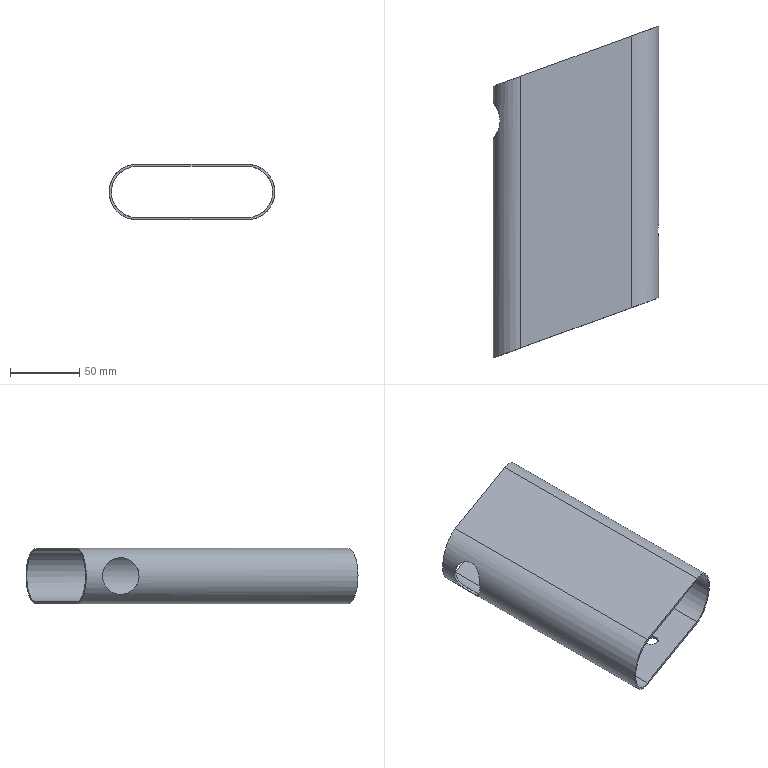Part | STEP file | Q7C0104R | 1 solid | 15 faces | box 120 x 240.549 x 40 mm | volume 81709 mm3 | cylinder 9 | plane 6 | commonest cylinder face diameters 10 x3 37 x2 40 x2 3.5 x1 26.5 x1